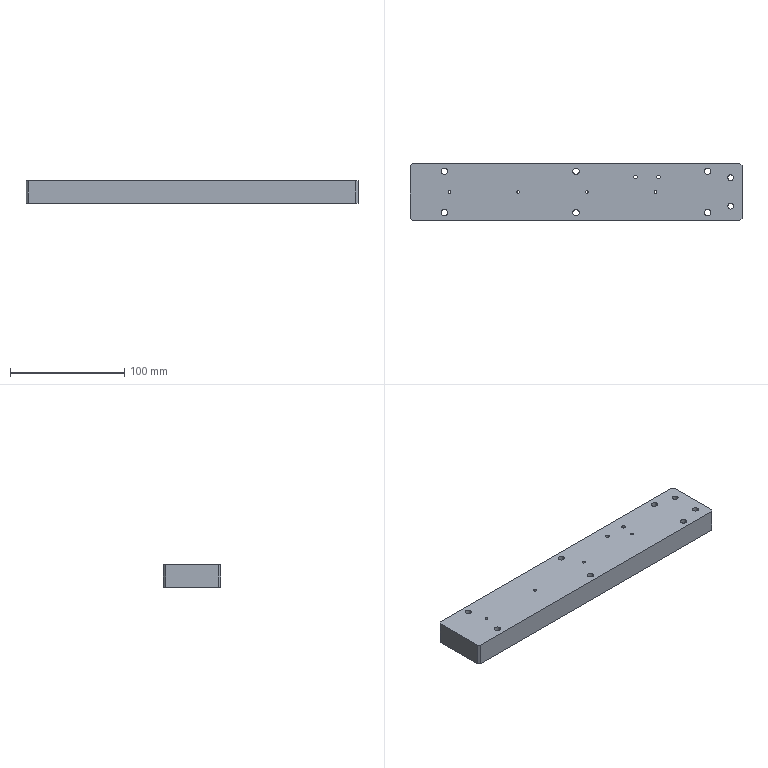Part | STEP file | FBDS-CS-012 | 1 solid | 60 faces | box 290 x 50 x 20 mm | volume 283331 mm3 | cylinder 40 | plane 16 | cone 4 | commonest cylinder face diameters 5.5 x12 10 x12 2.5 x8 3.3 x4 5 x4